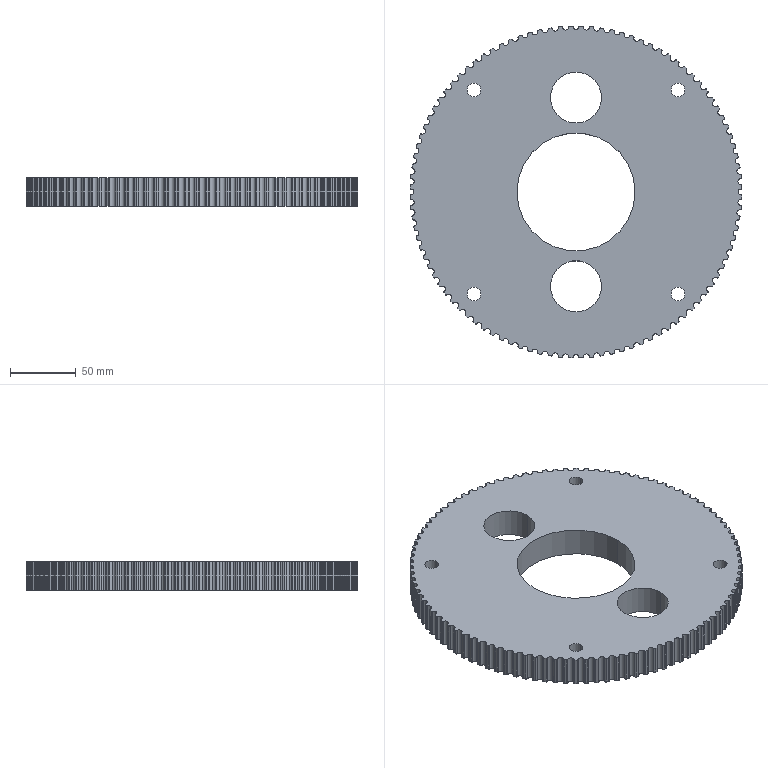Part | STEP file | Tube-changer large pulley SGN-2-09 | 1 solid | 711 faces | box 253.24 x 253.244 x 22 mm | volume 884088 mm3 | cylinder 410 | plane 301 | commonest cylinder face diameters 1.62 x248 4.57 x147 10.5 x8 39 x4 90 x2 30.218 x1